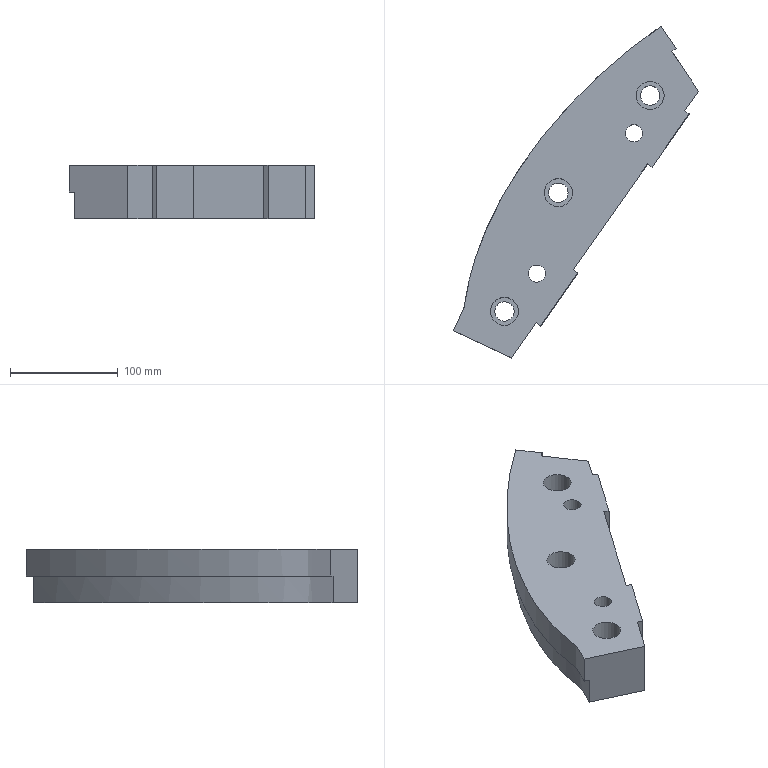Part | NX | features solid 2 | 1 solid | 29 faces | box 227.063 x 307.459 x 50 mm | volume 1256974 mm3 | plane 18 | cylinder 8 | spline 3 | commonest cylinder face diameters 18 x3 26 x3 16 x2
STEP:
#1=CARTESIAN_POINT('',(-702.221,92.253,-50.));
#2=VERTEX_POINT('',#1);
#3=CARTESIAN_POINT('',(-711.221,92.253,-50.));
#4=DIRECTION('',(0.,0.,1.));
#5=DIRECTION('',(1.,0.,0.));
#6=AXIS2_PLACEMENT_3D('',#3,#4,#5);
#7=CIRCLE('',#6,9.);
#8=EDGE_CURVE('',#2,#2,#7,.T.);
#9=ORIENTED_EDGE('',*,*,#8,.F.);
#10=EDGE_LOOP('',(#9));
#11=FACE_BOUND('',#10,.T.);
#12=CARTESIAN_POINT('',(-702.221,92.253,-30.));
#13=VERTEX_POINT('',#12);
#14=CARTESIAN_POINT('',(-711.221,92.253,-30.));
#15=DIRECTION('',(0.,0.,1.));
#16=DIRECTION('',(1.,0.,0.));
#17=AXIS2_PLACEMENT_3D('',#14,#15,#16);
#18=CIRCLE('',#17,9.);
#19=EDGE_CURVE('',#13,#13,#18,.F.);
#20=ORIENTED_EDGE('',*,*,#19,.F.);
#21=EDGE_LOOP('',(#20));
#22=FACE_BOUND('',#21,.T.);
#23=CARTESIAN_POINT('',(-711.221,92.253,-125.));
#24=DIRECTION('',(0.,0.,1.));
#25=DIRECTION('',(1.,0.,0.));
#26=AXIS2_PLACEMENT_3D('',#23,#24,#25);
#27=CYLINDRICAL_SURFACE('',#26,9.);
#28=ADVANCED_FACE('',(#11,#22),#27,.F.);
#29=CARTESIAN_POINT('',(-652.221,202.253,-50.));
#30=VERTEX_POINT('',#29);
#31=CARTESIAN_POINT('',(-661.221,202.253,-50.));
#32=DIRECTION('',(0.,0.,1.));
#33=DIRECTION('',(1.,0.,0.));
#34=AXIS2_PLACEMENT_3D('',#31,#32,#33);
#35=CIRCLE('',#34,9.);
#36=EDGE_CURVE('',#30,#30,#35,.T.);
#37=ORIENTED_EDGE('',*,*,#36,.F.);
#38=EDGE_LOOP('',(#37));
#39=FACE_BOUND('',#38,.T.);
#40=CARTESIAN_POINT('',(-652.221,202.253,-30.));
#41=VERTEX_POINT('',#40);
#42=CARTESIAN_POINT('',(-661.221,202.253,-30.));
#43=DIRECTION('',(0.,0.,1.));
#44=DIRECTION('',(1.,0.,0.));
#45=AXIS2_PLACEMENT_3D('',#42,#43,#44);
#46=CIRCLE('',#45,9.);
#47=EDGE_CURVE('',#41,#41,#46,.F.);
#48=ORIENTED_EDGE('',*,*,#47,.F.);
#49=EDGE_LOOP('',(#48));
#50=FACE_BOUND('',#49,.T.);
#51=CARTESIAN_POINT('',(-661.221,202.253,-125.));
#52=DIRECTION('',(0.,0.,1.));
#53=DIRECTION('',(1.,0.,0.));
#54=AXIS2_PLACEMENT_3D('',#51,#52,#53);
#55=CYLINDRICAL_SURFACE('',#54,9.);
#56=ADVANCED_FACE('',(#39,#50),#55,.F.);
#57=CARTESIAN_POINT('',(-567.221,292.253,-50.));
#58=VERTEX_POINT('',#57);
#59=CARTESIAN_POINT('',(-576.221,292.253,-50.));
#60=DIRECTION('',(0.,0.,1.));
#61=DIRECTION('',(1.,0.,0.));
#62=AXIS2_PLACEMENT_3D('',#59,#60,#61);
#63=CIRCLE('',#62,9.);
#64=EDGE_CURVE('',#58,#58,#63,.T.);
#65=ORIENTED_EDGE('',*,*,#64,.F.);
#66=EDGE_LOOP('',(#65));
#67=FACE_BOUND('',#66,.T.);
#68=CARTESIAN_POINT('',(-567.221,292.253,-30.));
#69=VERTEX_POINT('',#68);
#70=CARTESIAN_POINT('',(-576.221,292.253,-30.));
#71=DIRECTION('',(0.,0.,1.));
#72=DIRECTION('',(1.,0.,0.));
#73=AXIS2_PLACEMENT_3D('',#70,#71,#72);
#74=CIRCLE('',#73,9.);
#75=EDGE_CURVE('',#69,#69,#74,.F.);
#76=ORIENTED_EDGE('',*,*,#75,.F.);
#77=EDGE_LOOP('',(#76));
#78=FACE_BOUND('',#77,.T.);
#79=CARTESIAN_POINT('',(-576.221,292.253,-125.));
#80=DIRECTION('',(0.,0.,1.));
#81=DIRECTION('',(1.,0.,0.));
#82=AXIS2_PLACEMENT_3D('',#79,#80,#81);
#83=CYLINDRICAL_SURFACE('',#82,9.);
#84=ADVANCED_FACE('',(#67,#78),#83,.F.);
#85=CARTESIAN_POINT('',(-578.59,228.85,0.));
#86=VERTEX_POINT('',#85);
#87=CARTESIAN_POINT('',(-647.285,130.742,0.));
#88=VERTEX_POINT('',#87);
#89=CARTESIAN_POINT('',(-699.862,55.655,0.));
#90=DIRECTION('',(0.5736,0.8192,0.));
#91=VECTOR('',#90,1000.);
#92=LINE('',#89,#91);
#93=EDGE_CURVE('',#86,#88,#92,.F.);
#94=ORIENTED_EDGE('',*,*,#93,.T.);
#95=CARTESIAN_POINT('',(-647.285,130.742,-50.));
#96=VERTEX_POINT('',#95);
#97=CARTESIAN_POINT('',(-647.285,130.742,-70.));
#98=DIRECTION('',(0.,0.,-1.));
#99=VECTOR('',#98,1000.);
#100=LINE('',#97,#99);
#101=EDGE_CURVE('',#88,#96,#100,.T.);
#102=ORIENTED_EDGE('',*,*,#101,.T.);
#103=CARTESIAN_POINT('',(-578.59,228.85,-50.));
#104=VERTEX_POINT('',#103);
#105=CARTESIAN_POINT('',(-844.558,-150.992,-50.));
#106=DIRECTION('',(0.5736,0.8192,0.));
#107=VECTOR('',#106,1000.);
#108=LINE('',#105,#107);
#109=EDGE_CURVE('',#96,#104,#108,.T.);
#110=ORIENTED_EDGE('',*,*,#109,.T.);
#111=CARTESIAN_POINT('',(-578.59,228.85,-70.));
#112=DIRECTION('',(0.,0.,-1.));
#113=VECTOR('',#112,1000.);
#114=LINE('',#111,#113);
#115=EDGE_CURVE('',#86,#104,#114,.T.);
#116=ORIENTED_EDGE('',*,*,#115,.F.);
#117=EDGE_LOOP('',(#94,#102,#110,#116));
#118=FACE_BOUND('',#117,.T.);
#119=CARTESIAN_POINT('',(-705.68,47.346,-70.));
#120=DIRECTION('',(0.8192,-0.5736,0.));
#121=DIRECTION('',(0.5736,0.8192,0.));
#122=AXIS2_PLACEMENT_3D('',#119,#120,#121);
#123=PLANE('',#122);
#124=ADVANCED_FACE('',(#118),#123,.T.);
#125=CARTESIAN_POINT('',(-531.399,296.245,0.));
#126=VERTEX_POINT('',#125);
#127=CARTESIAN_POINT('',(-544.175,277.999,0.));
#128=VERTEX_POINT('',#127);
#129=CARTESIAN_POINT('',(-699.862,55.655,0.));
#130=DIRECTION('',(0.5736,0.8192,0.));
#131=VECTOR('',#130,1000.);
#132=LINE('',#129,#131);
#133=EDGE_CURVE('',#126,#128,#132,.F.);
#134=ORIENTED_EDGE('',*,*,#133,.T.);
#135=CARTESIAN_POINT('',(-544.175,277.999,-50.));
#136=VERTEX_POINT('',#135);
#137=CARTESIAN_POINT('',(-544.175,277.999,-70.));
#138=DIRECTION('',(0.,0.,-1.));
#139=VECTOR('',#138,1000.);
#140=LINE('',#137,#139);
#141=EDGE_CURVE('',#128,#136,#140,.T.);
#142=ORIENTED_EDGE('',*,*,#141,.T.);
#143=CARTESIAN_POINT('',(-531.399,296.245,-50.));
#144=VERTEX_POINT('',#143);
#145=CARTESIAN_POINT('',(-844.558,-150.992,-50.));
#146=DIRECTION('',(0.5736,0.8192,0.));
#147=VECTOR('',#146,1000.);
#148=LINE('',#145,#147);
#149=EDGE_CURVE('',#136,#144,#148,.T.);
#150=ORIENTED_EDGE('',*,*,#149,.T.);
#151=CARTESIAN_POINT('',(-531.399,296.245,-70.));
#152=DIRECTION('',(0.,0.,1.));
#153=VECTOR('',#152,1000.);
#154=LINE('',#151,#153);
#155=EDGE_CURVE('',#144,#126,#154,.T.);
#156=ORIENTED_EDGE('',*,*,#155,.T.);
#157=EDGE_LOOP('',(#134,#142,#150,#156));
#158=FACE_BOUND('',#157,.T.);
#159=CARTESIAN_POINT('',(-705.68,47.346,-70.));
#160=DIRECTION('',(0.8192,-0.5736,0.));
#161=DIRECTION('',(0.5736,0.8192,0.));
#162=AXIS2_PLACEMENT_3D('',#159,#160,#161);
#163=PLANE('',#162);
#164=ADVANCED_FACE('',(#158),#163,.T.);
#165=CARTESIAN_POINT('',(-567.378,349.586,-50.));
#166=VERTEX_POINT('',#165);
#167=CARTESIAN_POINT('',(-567.378,349.586,-25.));
#168=VERTEX_POINT('',#167);
#169=CARTESIAN_POINT('',(-567.378,349.586,-42.5));
#170=DIRECTION('',(0.,0.,1.));
#171=VECTOR('',#170,1000.);
#172=LINE('',#169,#171);
#173=EDGE_CURVE('',#166,#168,#172,.T.);
#174=ORIENTED_EDGE('',*,*,#173,.F.);
#175=CARTESIAN_POINT('',(-753.931,72.246,-50.));
#176=VERTEX_POINT('',#175);
#177=CARTESIAN_POINT('',(-753.931,72.246,-50.));
#178=CARTESIAN_POINT('',(-752.551,75.205,-50.));
#179=CARTESIAN_POINT('',(-750.712,79.146,-50.));
#180=CARTESIAN_POINT('',(-748.724,83.409,-50.));
#181=CARTESIAN_POINT('',(-747.464,86.109,-50.));
#182=CARTESIAN_POINT('',(-746.436,88.312,-50.));
#183=CARTESIAN_POINT('',(-745.772,89.735,-50.));
#184=CARTESIAN_POINT('',(-745.356,90.624,-50.));
#185=CARTESIAN_POINT('',(-745.145,91.076,-50.));
#186=CARTESIAN_POINT('',(-745.004,91.377,-50.));
#187=CARTESIAN_POINT('',(-744.914,91.569,-50.));
#188=CARTESIAN_POINT('',(-744.848,91.71,-50.));
#189=CARTESIAN_POINT('',(-744.815,91.781,-50.));
#190=CARTESIAN_POINT('',(-744.787,91.841,-50.));
#191=CARTESIAN_POINT('',(-744.797,91.819,-50.));
#192=CARTESIAN_POINT('',(-744.692,92.043,-50.));
#193=CARTESIAN_POINT('',(-744.597,92.252,-50.));
#194=CARTESIAN_POINT('',(-744.419,92.651,-50.));
#195=CARTESIAN_POINT('',(-744.109,93.399,-50.));
#196=CARTESIAN_POINT('',(-743.77,94.346,-50.));
#197=CARTESIAN_POINT('',(-743.446,95.594,-50.));
#198=CARTESIAN_POINT('',(-743.219,97.004,-50.));
#199=CARTESIAN_POINT('',(-743.024,98.542,-50.));
#200=CARTESIAN_POINT('',(-742.827,99.93,-50.));
#201=CARTESIAN_POINT('',(-742.634,101.268,-50.));
#202=CARTESIAN_POINT('',(-742.458,102.433,-50.));
#203=CARTESIAN_POINT('',(-742.239,103.818,-50.));
#204=CARTESIAN_POINT('',(-741.949,105.59,-50.));
#205=CARTESIAN_POINT('',(-741.559,107.839,-50.));
#206=CARTESIAN_POINT('',(-741.064,110.513,-50.));
#207=CARTESIAN_POINT('',(-740.519,113.264,-50.));
#208=CARTESIAN_POINT('',(-739.995,115.766,-50.));
#209=CARTESIAN_POINT('',(-739.238,119.196,-50.));
#210=CARTESIAN_POINT('',(-737.817,125.17,-50.));
#211=CARTESIAN_POINT('',(-735.949,132.044,-50.));
#212=CARTESIAN_POINT('',(-733.843,138.944,-50.));
#213=CARTESIAN_POINT('',(-732.145,144.128,-50.));
#214=CARTESIAN_POINT('',(-730.623,148.481,-50.));
#215=CARTESIAN_POINT('',(-729.362,151.925,-50.));
#216=CARTESIAN_POINT('',(-728.339,154.635,-50.));
#217=CARTESIAN_POINT('',(-727.468,156.882,-50.));
#218=CARTESIAN_POINT('',(-726.214,160.039,-50.));
#219=CARTESIAN_POINT('',(-724.611,163.93,-50.));
#220=CARTESIAN_POINT('',(-722.587,168.622,-50.));
#221=CARTESIAN_POINT('',(-719.77,174.869,-50.));
#222=CARTESIAN_POINT('',(-716.019,182.678,-50.));
#223=CARTESIAN_POINT('',(-711.153,192.044,-50.));
#224=CARTESIAN_POINT('',(-705.922,201.407,-50.));
#225=CARTESIAN_POINT('',(-700.323,210.77,-50.));
#226=CARTESIAN_POINT('',(-695.36,218.56,-50.));
#227=CARTESIAN_POINT('',(-691.712,224.03,-50.));
#228=CARTESIAN_POINT('',(-689.603,227.126,-50.));
#229=CARTESIAN_POINT('',(-687.94,229.531,-50.));
#230=CARTESIAN_POINT('',(-686.478,231.617,-50.));
#231=CARTESIAN_POINT('',(-684.43,234.502,-50.));
#232=CARTESIAN_POINT('',(-680.824,239.483,-50.));
#233=CARTESIAN_POINT('',(-675.492,246.575,-50.));
#234=CARTESIAN_POINT('',(-669.938,253.603,-50.));
#235=CARTESIAN_POINT('',(-665.38,259.168,-50.));
#236=CARTESIAN_POINT('',(-661.844,263.382,-50.));
#237=CARTESIAN_POINT('',(-658.443,267.345,-50.));
#238=CARTESIAN_POINT('',(-653.774,272.668,-50.));
#239=CARTESIAN_POINT('',(-647.828,279.227,-50.));
#240=CARTESIAN_POINT('',(-640.502,286.968,-50.));
#241=CARTESIAN_POINT('',(-632.883,294.678,-50.));
#242=CARTESIAN_POINT('',(-625.396,301.943,-50.));
#243=CARTESIAN_POINT('',(-615.06,311.564,-50.));
#244=CARTESIAN_POINT('',(-596.387,327.892,-50.));
#245=CARTESIAN_POINT('',(-579.271,341.12,-50.));
#246=CARTESIAN_POINT('',(-567.378,349.586,-50.));
#247=B_SPLINE_CURVE_WITH_KNOTS('',3,(#177,#178,#179,#180,#181,#182,#183,#184,#185,#186,#187,#188,#189,#190,#191,#192,#193,#194,#195,#196,#197,#198,#199,#200,#201,#202,#203,#204,#205,#206,#207,#208,#209,#210,#211,#212,#213,#214,#215,#216,#217,#218,#219,#220,#221,#222,#223,#224,#225,#226,#227,#228,#229,#230,#231,#232,#233,#234,#235,#236,#237,#238,#239,#240,#241,#242,#243,#244,#245,#246),.UNSPECIFIED.,.F.,.F.,(4,1,1,1,1,1,1,1,1,1,1,1,1,1,1,1,1,1,1,1,1,1,1,1,1,1,1,1,1,1,1,1,1,1,1,1,1,1,1,1,1,1,1,1,1,1,1,1,1,1,1,1,1,1,1,1,1,1,1,1,1,1,1,1,1,1,1,4),(0.,0.01562,0.02344,0.03125,0.03906,0.04688,0.05078,0.05469,0.05664,0.05859,0.06055,0.06152,0.06201,0.0625,0.06299,0.06348,0.06445,0.06641,0.07031,0.07422,0.07812,0.08203,0.08594,0.08984,0.09375,0.09766,0.1016,0.1094,0.1172,0.125,0.1328,0.1406,0.1562,0.1875,0.2031,0.2188,0.2344,0.2422,0.25,0.2578,0.2656,0.2812,0.2969,0.3125,0.3438,0.375,0.4062,0.4375,0.4688,0.4844,0.4922,0.5,0.5078,0.5156,0.5312,0.5625,0.5938,0.6094,0.625,0.6406,0.6562,0.6875,0.7188,0.75,0.7812,0.8125,0.875,1.),.UNSPECIFIED.);
#248=EDGE_CURVE('',#176,#166,#247,.T.);
#249=ORIENTED_EDGE('',*,*,#248,.F.);
#250=CARTESIAN_POINT('',(-753.931,72.246,-25.));
#251=VERTEX_POINT('',#250);
#252=CARTESIAN_POINT('',(-753.931,72.246,-42.5));
#253=DIRECTION('',(0.,0.,1.));
#254=VECTOR('',#253,1000.);
#255=LINE('',#252,#254);
#256=EDGE_CURVE('',#176,#251,#255,.T.);
#257=ORIENTED_EDGE('',*,*,#256,.T.);
#258=CARTESIAN_POINT('',(-567.378,349.586,-25.));
#259=CARTESIAN_POINT('',(-579.003,341.311,-25.));
#260=CARTESIAN_POINT('',(-601.651,323.884,-25.));
#261=CARTESIAN_POINT('',(-633.362,294.993,-25.));
#262=CARTESIAN_POINT('',(-657.503,268.971,-25.));
#263=CARTESIAN_POINT('',(-675.422,246.874,-25.));
#264=CARTESIAN_POINT('',(-688.122,229.581,-25.));
#265=CARTESIAN_POINT('',(-699.93,211.672,-25.));
#266=CARTESIAN_POINT('',(-710.667,193.273,-25.));
#267=CARTESIAN_POINT('',(-720.263,174.286,-25.));
#268=CARTESIAN_POINT('',(-728.596,154.68,-25.));
#269=CARTESIAN_POINT('',(-734.383,137.731,-25.));
#270=CARTESIAN_POINT('',(-738.192,123.83,-25.));
#271=CARTESIAN_POINT('',(-740.199,115.014,-25.));
#272=CARTESIAN_POINT('',(-741.571,107.876,-25.));
#273=CARTESIAN_POINT('',(-742.317,103.375,-25.));
#274=CARTESIAN_POINT('',(-742.867,99.758,-25.));
#275=CARTESIAN_POINT('',(-743.198,97.016,-25.));
#276=CARTESIAN_POINT('',(-743.685,94.33,-25.));
#277=CARTESIAN_POINT('',(-744.763,91.854,-25.));
#278=CARTESIAN_POINT('',(-745.932,89.412,-25.));
#279=CARTESIAN_POINT('',(-747.448,86.139,-25.));
#280=CARTESIAN_POINT('',(-749.358,82.054,-25.));
#281=CARTESIAN_POINT('',(-751.643,77.15,-25.));
#282=CARTESIAN_POINT('',(-753.168,73.88,-25.));
#283=CARTESIAN_POINT('',(-753.931,72.246,-25.));
#284=B_SPLINE_CURVE_WITH_KNOTS('',3,(#258,#259,#260,#261,#262,#263,#264,#265,#266,#267,#268,#269,#270,#271,#272,#273,#274,#275,#276,#277,#278,#279,#280,#281,#282,#283),.UNSPECIFIED.,.F.,.F.,(4,1,1,1,1,1,1,1,1,1,1,1,1,1,1,1,1,1,1,1,1,1,1,4),(0.7775,0.8203,0.8631,0.9059,0.9273,0.9487,0.9701,0.9916,1.013,1.034,1.056,1.066,1.077,1.083,1.088,1.091,1.093,1.096,1.099,1.101,1.104,1.109,1.115,1.12),.UNSPECIFIED.);
#285=EDGE_CURVE('',#251,#168,#284,.F.);
#286=ORIENTED_EDGE('',*,*,#285,.T.);
#287=EDGE_LOOP('',(#174,#249,#257,#286));
#288=FACE_BOUND('',#287,.T.);
#289=CARTESIAN_POINT('',(-753.931,72.246,-50.));
#290=CARTESIAN_POINT('',(-753.931,72.246,-25.));
#291=CARTESIAN_POINT('',(-753.17,73.877,-50.));
#292=CARTESIAN_POINT('',(-753.17,73.877,-25.));
#293=CARTESIAN_POINT('',(-751.649,77.139,-50.));
#294=CARTESIAN_POINT('',(-751.649,77.139,-25.));
#295=CARTESIAN_POINT('',(-749.747,81.217,-50.));
#296=CARTESIAN_POINT('',(-749.747,81.217,-25.));
#297=CARTESIAN_POINT('',(-748.226,84.48,-50.));
#298=CARTESIAN_POINT('',(-748.226,84.48,-25.));
#299=CARTESIAN_POINT('',(-747.275,86.518,-50.));
#300=CARTESIAN_POINT('',(-747.275,86.518,-25.));
#301=CARTESIAN_POINT('',(-746.514,88.151,-50.));
#302=CARTESIAN_POINT('',(-746.514,88.151,-25.));
#303=CARTESIAN_POINT('',(-745.946,89.367,-50.));
#304=CARTESIAN_POINT('',(-745.946,89.367,-25.));
#305=CARTESIAN_POINT('',(-745.367,90.611,-50.));
#306=CARTESIAN_POINT('',(-745.367,90.611,-25.));
#307=CARTESIAN_POINT('',(-744.842,91.716,-50.));
#308=CARTESIAN_POINT('',(-744.842,91.716,-25.));
#309=CARTESIAN_POINT('',(-744.099,93.332,-50.));
#310=CARTESIAN_POINT('',(-744.099,93.332,-25.));
#311=CARTESIAN_POINT('',(-743.469,95.313,-50.));
#312=CARTESIAN_POINT('',(-743.469,95.313,-25.));
#313=CARTESIAN_POINT('',(-743.227,96.983,-50.));
#314=CARTESIAN_POINT('',(-743.227,96.983,-25.));
#315=CARTESIAN_POINT('',(-743.125,97.786,-50.));
#316=CARTESIAN_POINT('',(-743.125,97.786,-25.));
#317=CARTESIAN_POINT('',(-743.005,98.675,-50.));
#318=CARTESIAN_POINT('',(-743.005,98.675,-25.));
#319=CARTESIAN_POINT('',(-742.855,99.756,-50.));
#320=CARTESIAN_POINT('',(-742.855,99.756,-25.));
#321=CARTESIAN_POINT('',(-742.601,101.501,-50.));
#322=CARTESIAN_POINT('',(-742.601,101.501,-25.));
#323=CARTESIAN_POINT('',(-742.266,103.673,-50.));
#324=CARTESIAN_POINT('',(-742.266,103.673,-25.));
#325=CARTESIAN_POINT('',(-741.833,106.278,-50.));
#326=CARTESIAN_POINT('',(-741.833,106.278,-25.));
#327=CARTESIAN_POINT('',(-741.216,109.745,-50.));
#328=CARTESIAN_POINT('',(-741.216,109.745,-25.));
#329=CARTESIAN_POINT('',(-740.369,114.065,-50.));
#330=CARTESIAN_POINT('',(-740.369,114.065,-25.));
#331=CARTESIAN_POINT('',(-739.238,119.229,-50.));
#332=CARTESIAN_POINT('',(-739.238,119.229,-25.));
#333=CARTESIAN_POINT('',(-737.579,126.085,-50.));
#334=CARTESIAN_POINT('',(-737.579,126.085,-25.));
#335=CARTESIAN_POINT('',(-735.232,134.596,-50.));
#336=CARTESIAN_POINT('',(-735.232,134.596,-25.));
#337=CARTESIAN_POINT('',(-732.002,144.701,-50.));
#338=CARTESIAN_POINT('',(-732.002,144.701,-25.));
#339=CARTESIAN_POINT('',(-727.177,158.017,-50.));
#340=CARTESIAN_POINT('',(-727.177,158.017,-25.));
#341=CARTESIAN_POINT('',(-720.244,174.327,-50.));
#342=CARTESIAN_POINT('',(-720.244,174.327,-25.));
#343=CARTESIAN_POINT('',(-710.641,193.322,-50.));
#344=CARTESIAN_POINT('',(-710.641,193.322,-25.));
#345=CARTESIAN_POINT('',(-699.889,211.737,-50.));
#346=CARTESIAN_POINT('',(-699.889,211.737,-25.));
#347=CARTESIAN_POINT('',(-684.216,235.503,-50.));
#348=CARTESIAN_POINT('',(-684.216,235.503,-25.));
#349=CARTESIAN_POINT('',(-662.409,263.684,-50.));
#350=CARTESIAN_POINT('',(-662.409,263.684,-25.));
#351=CARTESIAN_POINT('',(-623.582,305.544,-50.));
#352=CARTESIAN_POINT('',(-623.582,305.544,-25.));
#353=CARTESIAN_POINT('',(-590.637,333.029,-50.));
#354=CARTESIAN_POINT('',(-590.637,333.029,-25.));
#355=CARTESIAN_POINT('',(-567.378,349.586,-50.));
#356=CARTESIAN_POINT('',(-567.378,349.586,-25.));
#357=B_SPLINE_SURFACE_WITH_KNOTS('',3,1,((#289,#290),(#291,#292),(#293,#294),(#295,#296),(#297,#298),(#299,#300),(#301,#302),(#303,#304),(#305,#306),(#307,#308),(#309,#310),(#311,#312),(#313,#314),(#315,#316),(#317,#318),(#319,#320),(#321,#322),(#323,#324),(#325,#326),(#327,#328),(#329,#330),(#331,#332),(#333,#334),(#335,#336),(#337,#338),(#339,#340),(#341,#342),(#343,#344),(#345,#346),(#347,#348),(#349,#350),(#351,#352),(#353,#354),(#355,#356)),.SURF_OF_LINEAR_EXTRUSION.,.F.,.F.,.F.,(4,1,1,1,1,1,1,1,1,1,1,1,1,1,1,1,1,1,1,1,1,1,1,1,1,1,1,1,1,1,1,4),(2,2),(0.,0.0154,0.03079,0.03849,0.04619,0.05004,0.05389,0.05774,0.06159,0.06544,0.06928,0.07313,0.07506,0.07698,0.08083,0.08468,0.09238,0.1001,0.1078,0.1232,0.1386,0.154,0.1848,0.2156,0.2463,0.3079,0.3695,0.4311,0.4927,0.6159,0.739,0.9854),(0.,1.),.UNSPECIFIED.);
#358=ADVANCED_FACE('',(#288),#357,.F.);
#359=CARTESIAN_POINT('',(-704.413,49.155,-50.));
#360=VERTEX_POINT('',#359);
#361=CARTESIAN_POINT('',(-704.413,49.155,0.));
#362=VERTEX_POINT('',#361);
#363=CARTESIAN_POINT('',(-704.413,49.155,-70.));
#364=DIRECTION('',(0.,0.,1.));
#365=VECTOR('',#364,1000.);
#366=LINE('',#363,#365);
#367=EDGE_CURVE('',#360,#362,#366,.T.);
#368=ORIENTED_EDGE('',*,*,#367,.F.);
#369=CARTESIAN_POINT('',(-681.7,81.593,-50.));
#370=VERTEX_POINT('',#369);
#371=CARTESIAN_POINT('',(-844.558,-150.992,-50.));
#372=DIRECTION('',(0.5736,0.8192,0.));
#373=VECTOR('',#372,1000.);
#374=LINE('',#371,#373);
#375=EDGE_CURVE('',#360,#370,#374,.T.);
#376=ORIENTED_EDGE('',*,*,#375,.T.);
#377=CARTESIAN_POINT('',(-681.7,81.593,0.));
#378=VERTEX_POINT('',#377);
#379=CARTESIAN_POINT('',(-681.7,81.593,-70.));
#380=DIRECTION('',(0.,0.,-1.));
#381=VECTOR('',#380,1000.);
#382=LINE('',#379,#381);
#383=EDGE_CURVE('',#378,#370,#382,.T.);
#384=ORIENTED_EDGE('',*,*,#383,.F.);
#385=CARTESIAN_POINT('',(-699.862,55.655,0.));
#386=DIRECTION('',(0.5736,0.8192,0.));
#387=VECTOR('',#386,1000.);
#388=LINE('',#385,#387);
#389=EDGE_CURVE('',#378,#362,#388,.F.);
#390=ORIENTED_EDGE('',*,*,#389,.T.);
#391=EDGE_LOOP('',(#368,#376,#384,#390));
#392=FACE_BOUND('',#391,.T.);
#393=CARTESIAN_POINT('',(-705.68,47.346,-70.));
#394=DIRECTION('',(0.8192,-0.5736,0.));
#395=DIRECTION('',(0.5736,0.8192,0.));
#396=AXIS2_PLACEMENT_3D('',#393,#394,#395);
#397=PLANE('',#396);
#398=ADVANCED_FACE('',(#392),#397,.T.);
#399=CARTESIAN_POINT('',(-552.106,335.885,-25.));
#400=VERTEX_POINT('',#399);
#401=CARTESIAN_POINT('',(-552.106,335.885,0.));
#402=VERTEX_POINT('',#401);
#403=CARTESIAN_POINT('',(-552.106,335.885,-12.5));
#404=DIRECTION('',(0.,0.,-1.));
#405=VECTOR('',#404,1000.);
#406=LINE('',#403,#405);
#407=EDGE_CURVE('',#400,#402,#406,.F.);
#408=ORIENTED_EDGE('',*,*,#407,.F.);
#409=CARTESIAN_POINT('',(-566.088,356.614,-25.));
#410=VERTEX_POINT('',#409);
#411=CARTESIAN_POINT('',(822.371,-1701.861,-25.));
#412=DIRECTION('',(-0.5592,0.829,0.));
#413=VECTOR('',#412,1000.);
#414=LINE('',#411,#413);
#415=EDGE_CURVE('',#400,#410,#414,.T.);
#416=ORIENTED_EDGE('',*,*,#415,.T.);
#417=CARTESIAN_POINT('',(-566.088,356.614,0.));
#418=VERTEX_POINT('',#417);
#419=CARTESIAN_POINT('',(-566.088,356.614,-70.));
#420=DIRECTION('',(0.,0.,1.));
#421=VECTOR('',#420,1000.);
#422=LINE('',#419,#421);
#423=EDGE_CURVE('',#410,#418,#422,.T.);
#424=ORIENTED_EDGE('',*,*,#423,.T.);
#425=CARTESIAN_POINT('',(822.371,-1701.861,0.));
#426=DIRECTION('',(0.5592,-0.829,0.));
#427=VECTOR('',#426,1000.);
#428=LINE('',#425,#427);
#429=EDGE_CURVE('',#402,#418,#428,.F.);
#430=ORIENTED_EDGE('',*,*,#429,.F.);
#431=EDGE_LOOP('',(#408,#416,#424,#430));
#432=FACE_BOUND('',#431,.T.);
#433=CARTESIAN_POINT('',(822.371,-1701.861,-70.));
#434=DIRECTION('',(0.829,0.5592,0.));
#435=DIRECTION('',(-0.5592,0.829,0.));
#436=AXIS2_PLACEMENT_3D('',#433,#434,#435);
#437=PLANE('',#436);
#438=ADVANCED_FACE('',(#432),#437,.T.);
#439=ORIENTED_EDGE('',*,*,#8,.T.);
#440=EDGE_LOOP('',(#439));
#441=FACE_BOUND('',#440,.T.);
#442=CARTESIAN_POINT('',(-673.221,127.253,-50.));
#443=VERTEX_POINT('',#442);
#444=CARTESIAN_POINT('',(-681.221,127.253,-50.));
#445=DIRECTION('',(0.,0.,1.));
#446=DIRECTION('',(1.,0.,0.));
#447=AXIS2_PLACEMENT_3D('',#444,#445,#446);
#448=CIRCLE('',#447,8.);
#449=EDGE_CURVE('',#443,#443,#448,.T.);
#450=ORIENTED_EDGE('',*,*,#449,.T.);
#451=EDGE_LOOP('',(#450));
#452=FACE_BOUND('',#451,.T.);
#453=ORIENTED_EDGE('',*,*,#36,.T.);
#454=EDGE_LOOP('',(#453));
#455=FACE_BOUND('',#454,.T.);
#456=CARTESIAN_POINT('',(-583.221,257.253,-50.));
#457=VERTEX_POINT('',#456);
#458=CARTESIAN_POINT('',(-591.221,257.253,-50.));
#459=DIRECTION('',(0.,0.,1.));
#460=DIRECTION('',(1.,0.,0.));
#461=AXIS2_PLACEMENT_3D('',#458,#459,#460);
#462=CIRCLE('',#461,8.);
#463=EDGE_CURVE('',#457,#457,#462,.T.);
#464=ORIENTED_EDGE('',*,*,#463,.T.);
#465=EDGE_LOOP('',(#464));
#466=FACE_BOUND('',#465,.T.);
#467=ORIENTED_EDGE('',*,*,#64,.T.);
#468=EDGE_LOOP('',(#467));
#469=FACE_BOUND('',#468,.T.);
#470=ORIENTED_EDGE('',*,*,#375,.F.);
#471=CARTESIAN_POINT('',(-752.052,71.37,-50.));
#472=DIRECTION('',(0.9063,-0.4226,0.));
#473=VECTOR('',#472,1000.);
#474=LINE('',#471,#473);
#475=EDGE_CURVE('',#176,#360,#474,.T.);
#476=ORIENTED_EDGE('',*,*,#475,.F.);
#477=ORIENTED_EDGE('',*,*,#248,.T.);
#478=CARTESIAN_POINT('',(-427.361,142.001,-50.));
#479=DIRECTION('',(-0.5592,0.829,0.));
#480=VECTOR('',#479,1000.);
#481=LINE('',#478,#480);
#482=EDGE_CURVE('',#144,#166,#481,.T.);
#483=ORIENTED_EDGE('',*,*,#482,.F.);
#484=ORIENTED_EDGE('',*,*,#149,.F.);
#485=CARTESIAN_POINT('',(-540.079,275.131,-50.));
#486=VERTEX_POINT('',#485);
#487=CARTESIAN_POINT('',(-527.792,266.527,-50.));
#488=DIRECTION('',(0.8192,-0.5736,0.));
#489=VECTOR('',#488,1000.);
#490=LINE('',#487,#489);
#491=EDGE_CURVE('',#136,#486,#490,.T.);
#492=ORIENTED_EDGE('',*,*,#491,.T.);
#493=CARTESIAN_POINT('',(-574.494,225.982,-50.));
#494=VERTEX_POINT('',#493);
#495=CARTESIAN_POINT('',(-840.462,-153.86,-50.));
#496=DIRECTION('',(0.5736,0.8192,0.));
#497=VECTOR('',#496,1000.);
#498=LINE('',#495,#497);
#499=EDGE_CURVE('',#494,#486,#498,.T.);
#500=ORIENTED_EDGE('',*,*,#499,.F.);
#501=CARTESIAN_POINT('',(-562.206,217.378,-50.));
#502=DIRECTION('',(0.8192,-0.5736,0.));
#503=VECTOR('',#502,1000.);
#504=LINE('',#501,#503);
#505=EDGE_CURVE('',#104,#494,#504,.T.);
#506=ORIENTED_EDGE('',*,*,#505,.F.);
#507=ORIENTED_EDGE('',*,*,#109,.F.);
#508=CARTESIAN_POINT('',(-643.19,127.874,-50.));
#509=VERTEX_POINT('',#508);
#510=CARTESIAN_POINT('',(-630.902,119.27,-50.));
#511=DIRECTION('',(0.8192,-0.5736,0.));
#512=VECTOR('',#511,1000.);
#513=LINE('',#510,#512);
#514=EDGE_CURVE('',#96,#509,#513,.T.);
#515=ORIENTED_EDGE('',*,*,#514,.T.);
#516=CARTESIAN_POINT('',(-677.604,78.725,-50.));
#517=VERTEX_POINT('',#516);
#518=CARTESIAN_POINT('',(-840.462,-153.86,-50.));
#519=DIRECTION('',(0.5736,0.8192,0.));
#520=VECTOR('',#519,1000.);
#521=LINE('',#518,#520);
#522=EDGE_CURVE('',#517,#509,#521,.T.);
#523=ORIENTED_EDGE('',*,*,#522,.F.);
#524=CARTESIAN_POINT('',(-665.317,70.121,-50.));
#525=DIRECTION('',(0.8192,-0.5736,0.));
#526=VECTOR('',#525,1000.);
#527=LINE('',#524,#526);
#528=EDGE_CURVE('',#370,#517,#527,.T.);
#529=ORIENTED_EDGE('',*,*,#528,.F.);
#530=EDGE_LOOP('',(#470,#476,#477,#483,#484,#492,#500,#506,#507,#515,#523,#529));
#531=FACE_BOUND('',#530,.T.);
#532=CARTESIAN_POINT('',(-852.989,-145.089,-50.));
#533=DIRECTION('',(0.,0.,1.));
#534=DIRECTION('',(1.,0.,0.));
#535=AXIS2_PLACEMENT_3D('',#532,#533,#534);
#536=PLANE('',#535);
#537=ADVANCED_FACE('',(#441,#452,#455,#466,#469,#531),#536,.F.);
#538=CARTESIAN_POINT('',(-758.462,74.359,0.));
#539=VERTEX_POINT('',#538);
#540=CARTESIAN_POINT('',(-2805.507,1028.912,0.));
#541=DIRECTION('',(-0.9063,0.4226,0.));
#542=VECTOR('',#541,1000.);
#543=LINE('',#540,#542);
#544=EDGE_CURVE('',#539,#362,#543,.F.);
#545=ORIENTED_EDGE('',*,*,#544,.T.);
#546=ORIENTED_EDGE('',*,*,#389,.F.);
#547=CARTESIAN_POINT('',(-677.604,78.725,0.));
#548=VERTEX_POINT('',#547);
#549=CARTESIAN_POINT('',(-735.627,119.353,0.));
#550=DIRECTION('',(0.8192,-0.5736,0.));
#551=VECTOR('',#550,1000.);
#552=LINE('',#549,#551);
#553=EDGE_CURVE('',#378,#548,#552,.T.);
#554=ORIENTED_EDGE('',*,*,#553,.T.);
#555=CARTESIAN_POINT('',(-643.19,127.874,0.));
#556=VERTEX_POINT('',#555);
#557=CARTESIAN_POINT('',(-683.34,70.533,0.));
#558=DIRECTION('',(-0.5736,-0.8192,0.));
#559=VECTOR('',#558,1000.);
#560=LINE('',#557,#559);
#561=EDGE_CURVE('',#548,#556,#560,.F.);
#562=ORIENTED_EDGE('',*,*,#561,.T.);
#563=CARTESIAN_POINT('',(-701.212,168.502,0.));
#564=DIRECTION('',(0.8192,-0.5736,0.));
#565=VECTOR('',#564,1000.);
#566=LINE('',#563,#565);
#567=EDGE_CURVE('',#88,#556,#566,.T.);
#568=ORIENTED_EDGE('',*,*,#567,.F.);
#569=ORIENTED_EDGE('',*,*,#93,.F.);
#570=CARTESIAN_POINT('',(-574.494,225.982,0.));
#571=VERTEX_POINT('',#570);
#572=CARTESIAN_POINT('',(-632.516,266.61,0.));
#573=DIRECTION('',(0.8192,-0.5736,0.));
#574=VECTOR('',#573,1000.);
#575=LINE('',#572,#574);
#576=EDGE_CURVE('',#86,#571,#575,.T.);
#577=ORIENTED_EDGE('',*,*,#576,.T.);
#578=CARTESIAN_POINT('',(-540.079,275.131,0.));
#579=VERTEX_POINT('',#578);
#580=CARTESIAN_POINT('',(-563.022,242.365,0.));
#581=DIRECTION('',(-0.5736,-0.8192,0.));
#582=VECTOR('',#581,1000.);
#583=LINE('',#580,#582);
#584=EDGE_CURVE('',#571,#579,#583,.F.);
#585=ORIENTED_EDGE('',*,*,#584,.T.);
#586=CARTESIAN_POINT('',(-598.102,315.759,0.));
#587=DIRECTION('',(0.8192,-0.5736,0.));
#588=VECTOR('',#587,1000.);
#589=LINE('',#586,#588);
#590=EDGE_CURVE('',#128,#579,#589,.T.);
#591=ORIENTED_EDGE('',*,*,#590,.F.);
#592=ORIENTED_EDGE('',*,*,#133,.F.);
#593=CARTESIAN_POINT('',(-556.191,333.,0.));
#594=VERTEX_POINT('',#593);
#595=CARTESIAN_POINT('',(-509.098,263.181,0.));
#596=DIRECTION('',(-0.5592,0.829,0.));
#597=VECTOR('',#596,1000.);
#598=LINE('',#595,#597);
#599=EDGE_CURVE('',#126,#594,#598,.T.);
#600=ORIENTED_EDGE('',*,*,#599,.T.);
#601=CARTESIAN_POINT('',(-556.191,333.,0.));
#602=CARTESIAN_POINT('',(-554.834,333.967,0.));
#603=CARTESIAN_POINT('',(-553.472,334.93,0.));
#604=CARTESIAN_POINT('',(-552.106,335.885,0.));
#605=B_SPLINE_CURVE_WITH_KNOTS('',3,(#601,#602,#603,#604),.UNSPECIFIED.,.F.,.F.,(4,4),(1.826,1.831),.UNSPECIFIED.);
#606=EDGE_CURVE('',#594,#402,#605,.T.);
#607=ORIENTED_EDGE('',*,*,#606,.T.);
#608=ORIENTED_EDGE('',*,*,#429,.T.);
#609=CARTESIAN_POINT('',(-758.462,74.359,0.));
#610=CARTESIAN_POINT('',(-757.693,76.008,0.));
#611=CARTESIAN_POINT('',(-756.154,79.307,0.));
#612=CARTESIAN_POINT('',(-753.849,84.257,0.));
#613=CARTESIAN_POINT('',(-751.918,88.376,0.));
#614=CARTESIAN_POINT('',(-750.397,91.683,0.));
#615=CARTESIAN_POINT('',(-749.188,94.133,0.));
#616=CARTESIAN_POINT('',(-748.211,96.686,0.));
#617=CARTESIAN_POINT('',(-747.963,99.564,0.));
#618=CARTESIAN_POINT('',(-747.525,102.357,0.));
#619=CARTESIAN_POINT('',(-746.662,107.949,0.));
#620=CARTESIAN_POINT('',(-745.091,116.214,0.));
#621=CARTESIAN_POINT('',(-742.538,127.03,0.));
#622=CARTESIAN_POINT('',(-739.538,137.646,0.));
#623=CARTESIAN_POINT('',(-736.129,148.08,0.));
#624=CARTESIAN_POINT('',(-731.068,161.763,0.));
#625=CARTESIAN_POINT('',(-723.835,178.462,0.));
#626=CARTESIAN_POINT('',(-713.833,197.913,0.));
#627=CARTESIAN_POINT('',(-702.617,216.817,0.));
#628=CARTESIAN_POINT('',(-686.151,241.379,0.));
#629=CARTESIAN_POINT('',(-663.608,269.984,0.));
#630=CARTESIAN_POINT('',(-623.873,312.129,0.));
#631=CARTESIAN_POINT('',(-590.167,339.79,0.));
#632=CARTESIAN_POINT('',(-566.088,356.614,0.));
#633=B_SPLINE_CURVE_WITH_KNOTS('',3,(#609,#610,#611,#612,#613,#614,#615,#616,#617,#618,#619,#620,#621,#622,#623,#624,#625,#626,#627,#628,#629,#630,#631,#632),.UNSPECIFIED.,.F.,.F.,(4,1,1,1,1,1,1,1,1,1,1,1,1,1,1,1,1,1,1,1,1,4),(1.698,1.704,1.709,1.715,1.718,1.72,1.723,1.726,1.728,1.731,1.742,1.753,1.764,1.775,1.786,1.808,1.83,1.851,1.873,1.917,1.961,2.048),.UNSPECIFIED.);
#634=EDGE_CURVE('',#539,#418,#633,.T.);
#635=ORIENTED_EDGE('',*,*,#634,.F.);
#636=EDGE_LOOP('',(#545,#546,#554,#562,#568,#569,#577,#585,#591,#592,#600,#607,#608,#635));
#637=FACE_BOUND('',#636,.T.);
#638=CARTESIAN_POINT('',(-698.221,92.253,0.));
#639=VERTEX_POINT('',#638);
#640=CARTESIAN_POINT('',(-711.221,92.253,0.));
#641=DIRECTION('',(0.,0.,1.));
#642=DIRECTION('',(1.,0.,0.));
#643=AXIS2_PLACEMENT_3D('',#640,#641,#642);
#644=CIRCLE('',#643,13.);
#645=EDGE_CURVE('',#639,#639,#644,.T.);
#646=ORIENTED_EDGE('',*,*,#645,.F.);
#647=EDGE_LOOP('',(#646));
#648=FACE_BOUND('',#647,.T.);
#649=CARTESIAN_POINT('',(-648.221,202.253,0.));
#650=VERTEX_POINT('',#649);
#651=CARTESIAN_POINT('',(-661.221,202.253,0.));
#652=DIRECTION('',(0.,0.,1.));
#653=DIRECTION('',(1.,0.,0.));
#654=AXIS2_PLACEMENT_3D('',#651,#652,#653);
#655=CIRCLE('',#654,13.);
#656=EDGE_CURVE('',#650,#650,#655,.T.);
#657=ORIENTED_EDGE('',*,*,#656,.F.);
#658=EDGE_LOOP('',(#657));
#659=FACE_BOUND('',#658,.T.);
#660=CARTESIAN_POINT('',(-563.221,292.253,0.));
#661=VERTEX_POINT('',#660);
#662=CARTESIAN_POINT('',(-576.221,292.253,0.));
#663=DIRECTION('',(0.,0.,1.));
#664=DIRECTION('',(1.,0.,0.));
#665=AXIS2_PLACEMENT_3D('',#662,#663,#664);
#666=CIRCLE('',#665,13.);
#667=EDGE_CURVE('',#661,#661,#666,.T.);
#668=ORIENTED_EDGE('',*,*,#667,.F.);
#669=EDGE_LOOP('',(#668));
#670=FACE_BOUND('',#669,.T.);
#671=CARTESIAN_POINT('',(-673.221,127.253,0.));
#672=VERTEX_POINT('',#671);
#673=CARTESIAN_POINT('',(-681.221,127.253,0.));
#674=DIRECTION('',(0.,0.,1.));
#675=DIRECTION('',(1.,0.,0.));
#676=AXIS2_PLACEMENT_3D('',#673,#674,#675);
#677=CIRCLE('',#676,8.);
#678=EDGE_CURVE('',#672,#672,#677,.T.);
#679=ORIENTED_EDGE('',*,*,#678,.F.);
#680=EDGE_LOOP('',(#679));
#681=FACE_BOUND('',#680,.T.);
#682=CARTESIAN_POINT('',(-583.221,257.253,0.));
#683=VERTEX_POINT('',#682);
#684=CARTESIAN_POINT('',(-591.221,257.253,0.));
#685=DIRECTION('',(0.,0.,1.));
#686=DIRECTION('',(1.,0.,0.));
#687=AXIS2_PLACEMENT_3D('',#684,#685,#686);
#688=CIRCLE('',#687,8.);
#689=EDGE_CURVE('',#683,#683,#688,.T.);
#690=ORIENTED_EDGE('',*,*,#689,.F.);
#691=EDGE_LOOP('',(#690));
#692=FACE_BOUND('',#691,.T.);
#693=CARTESIAN_POINT('',(-663.,29.844,0.));
#694=DIRECTION('',(0.,0.,1.));
#695=DIRECTION('',(0.5736,0.8192,0.));
#696=AXIS2_PLACEMENT_3D('',#693,#694,#695);
#697=PLANE('',#696);
#698=ADVANCED_FACE('',(#637,#648,#659,#670,#681,#692),#697,.T.);
#699=CARTESIAN_POINT('',(-758.462,74.359,-25.));
#700=VERTEX_POINT('',#699);
#701=CARTESIAN_POINT('',(-758.462,74.359,-25.));
#702=CARTESIAN_POINT('',(-757.695,76.003,-25.));
#703=CARTESIAN_POINT('',(-756.161,79.292,-25.));
#704=CARTESIAN_POINT('',(-753.863,84.227,-25.));
#705=CARTESIAN_POINT('',(-751.938,88.335,-25.));
#706=CARTESIAN_POINT('',(-750.42,91.631,-25.));
#707=CARTESIAN_POINT('',(-749.22,94.076,-25.));
#708=CARTESIAN_POINT('',(-748.223,96.611,-25.));
#709=CARTESIAN_POINT('',(-747.973,99.481,-25.));
#710=CARTESIAN_POINT('',(-747.538,102.268,-25.));
#711=CARTESIAN_POINT('',(-746.68,107.846,-25.));
#712=CARTESIAN_POINT('',(-745.117,116.09,-25.));
#713=CARTESIAN_POINT('',(-742.577,126.879,-25.));
#714=CARTESIAN_POINT('',(-739.592,137.469,-25.));
#715=CARTESIAN_POINT('',(-736.199,147.877,-25.));
#716=CARTESIAN_POINT('',(-731.163,161.525,-25.));
#717=CARTESIAN_POINT('',(-723.966,178.181,-25.));
#718=CARTESIAN_POINT('',(-714.013,197.585,-25.));
#719=CARTESIAN_POINT('',(-702.859,216.433,-25.));
#720=CARTESIAN_POINT('',(-690.555,234.835,-25.));
#721=CARTESIAN_POINT('',(-677.333,252.572,-25.));
#722=CARTESIAN_POINT('',(-658.761,275.124,-25.));
#723=CARTESIAN_POINT('',(-633.84,301.556,-25.));
#724=CARTESIAN_POINT('',(-601.406,330.599,-25.));
#725=CARTESIAN_POINT('',(-578.115,348.211,-25.));
#726=CARTESIAN_POINT('',(-566.088,356.614,-25.));
#727=B_SPLINE_CURVE_WITH_KNOTS('',3,(#701,#702,#703,#704,#705,#706,#707,#708,#709,#710,#711,#712,#713,#714,#715,#716,#717,#718,#719,#720,#721,#722,#723,#724,#725,#726),.UNSPECIFIED.,.F.,.F.,(4,1,1,1,1,1,1,1,1,1,1,1,1,1,1,1,1,1,1,1,1,1,1,4),(1.367,1.372,1.378,1.383,1.386,1.389,1.392,1.394,1.397,1.4,1.411,1.421,1.432,1.443,1.454,1.476,1.498,1.519,1.541,1.563,1.585,1.628,1.672,1.715),.UNSPECIFIED.);
#728=EDGE_CURVE('',#700,#410,#727,.T.);
#729=ORIENTED_EDGE('',*,*,#728,.F.);
#730=CARTESIAN_POINT('',(-758.462,74.359,-2.5));
#731=DIRECTION('',(0.,0.,1.));
#732=VECTOR('',#731,1000.);
#733=LINE('',#730,#732);
#734=EDGE_CURVE('',#700,#539,#733,.T.);
#735=ORIENTED_EDGE('',*,*,#734,.T.);
#736=ORIENTED_EDGE('',*,*,#634,.T.);
#737=ORIENTED_EDGE('',*,*,#423,.F.);
#738=EDGE_LOOP('',(#729,#735,#736,#737));
#739=FACE_BOUND('',#738,.T.);
#740=CARTESIAN_POINT('',(-758.462,74.359,-25.));
#741=CARTESIAN_POINT('',(-758.462,74.359,0.));
#742=CARTESIAN_POINT('',(-757.69,76.014,-25.));
#743=CARTESIAN_POINT('',(-757.69,76.014,0.));
#744=CARTESIAN_POINT('',(-756.146,79.325,-25.));
#745=CARTESIAN_POINT('',(-756.146,79.325,0.));
#746=CARTESIAN_POINT('',(-753.833,84.292,-25.));
#747=CARTESIAN_POINT('',(-753.833,84.292,0.));
#748=CARTESIAN_POINT('',(-751.894,88.426,-25.));
#749=CARTESIAN_POINT('',(-751.894,88.426,0.));
#750=CARTESIAN_POINT('',(-750.368,91.746,-25.));
#751=CARTESIAN_POINT('',(-750.368,91.746,0.));
#752=CARTESIAN_POINT('',(-749.156,94.202,-25.));
#753=CARTESIAN_POINT('',(-749.156,94.202,0.));
#754=CARTESIAN_POINT('',(-748.335,96.346,-25.));
#755=CARTESIAN_POINT('',(-748.335,96.346,0.));
#756=CARTESIAN_POINT('',(-748.122,98.166,-25.));
#757=CARTESIAN_POINT('',(-748.122,98.166,0.));
#758=CARTESIAN_POINT('',(-747.749,100.878,-25.));
#759=CARTESIAN_POINT('',(-747.749,100.878,0.));
#760=CARTESIAN_POINT('',(-746.875,106.749,-25.));
#761=CARTESIAN_POINT('',(-746.875,106.749,0.));
#762=CARTESIAN_POINT('',(-745.194,115.721,-25.));
#763=CARTESIAN_POINT('',(-745.194,115.721,0.));
#764=CARTESIAN_POINT('',(-742.701,126.389,-25.));
#765=CARTESIAN_POINT('',(-742.701,126.389,0.));
#766=CARTESIAN_POINT('',(-739.751,136.946,-25.));
#767=CARTESIAN_POINT('',(-739.751,136.946,0.));
#768=CARTESIAN_POINT('',(-736.373,147.378,-25.));
#769=CARTESIAN_POINT('',(-736.373,147.378,0.));
#770=CARTESIAN_POINT('',(-731.333,161.108,-25.));
#771=CARTESIAN_POINT('',(-731.333,161.108,0.));
#772=CARTESIAN_POINT('',(-724.106,177.894,-25.));
#773=CARTESIAN_POINT('',(-724.106,177.894,0.));
#774=CARTESIAN_POINT('',(-710.781,203.911,-25.));
#775=CARTESIAN_POINT('',(-710.781,203.911,0.));
#776=CARTESIAN_POINT('',(-691.218,234.848,-25.));
#777=CARTESIAN_POINT('',(-691.218,234.848,0.));
#778=CARTESIAN_POINT('',(-664.149,269.379,-25.));
#779=CARTESIAN_POINT('',(-664.149,269.379,0.));
#780=CARTESIAN_POINT('',(-624.057,312.004,-25.));
#781=CARTESIAN_POINT('',(-624.057,312.004,0.));
#782=CARTESIAN_POINT('',(-590.047,339.875,-25.));
#783=CARTESIAN_POINT('',(-590.047,339.875,0.));
#784=CARTESIAN_POINT('',(-566.088,356.614,-25.));
#785=CARTESIAN_POINT('',(-566.088,356.614,0.));
#786=B_SPLINE_SURFACE_WITH_KNOTS('',3,1,((#740,#741),(#742,#743),(#744,#745),(#746,#747),(#748,#749),(#750,#751),(#752,#753),(#754,#755),(#756,#757),(#758,#759),(#760,#761),(#762,#763),(#764,#765),(#766,#767),(#768,#769),(#770,#771),(#772,#773),(#774,#775),(#776,#777),(#778,#779),(#780,#781),(#782,#783),(#784,#785)),.SURF_OF_LINEAR_EXTRUSION.,.F.,.F.,.F.,(4,1,1,1,1,1,1,1,1,1,1,1,1,1,1,1,1,1,1,1,4),(2,2),(0.003106,0.007784,0.01246,0.01714,0.01948,0.02182,0.02416,0.02533,0.02649,0.03117,0.04053,0.04988,0.05924,0.06859,0.07795,0.09666,0.1154,0.1528,0.1902,0.2276,0.3025),(0.,1.),.UNSPECIFIED.);
#787=ADVANCED_FACE('',(#739),#786,.F.);
#788=ORIENTED_EDGE('',*,*,#475,.T.);
#789=ORIENTED_EDGE('',*,*,#367,.T.);
#790=ORIENTED_EDGE('',*,*,#544,.F.);
#791=ORIENTED_EDGE('',*,*,#734,.F.);
#792=CARTESIAN_POINT('',(-758.462,74.359,-25.));
#793=DIRECTION('',(-0.9063,0.4226,0.));
#794=VECTOR('',#793,1000.);
#795=LINE('',#792,#794);
#796=EDGE_CURVE('',#251,#700,#795,.T.);
#797=ORIENTED_EDGE('',*,*,#796,.F.);
#798=ORIENTED_EDGE('',*,*,#256,.F.);
#799=EDGE_LOOP('',(#788,#789,#790,#791,#797,#798));
#800=FACE_BOUND('',#799,.T.);
#801=CARTESIAN_POINT('',(-2805.507,1028.912,-70.));
#802=DIRECTION('',(-0.4226,-0.9063,0.));
#803=DIRECTION('',(0.9063,-0.4226,0.));
#804=AXIS2_PLACEMENT_3D('',#801,#802,#803);
#805=PLANE('',#804);
#806=ADVANCED_FACE('',(#800),#805,.T.);
#807=ORIENTED_EDGE('',*,*,#415,.F.);
#808=CARTESIAN_POINT('',(-556.191,333.,-25.));
#809=VERTEX_POINT('',#808);
#810=CARTESIAN_POINT('',(-556.191,333.,-25.));
#811=CARTESIAN_POINT('',(-554.834,333.967,-25.));
#812=CARTESIAN_POINT('',(-553.473,334.929,-25.));
#813=CARTESIAN_POINT('',(-552.106,335.885,-25.));
#814=B_SPLINE_CURVE_WITH_KNOTS('',3,(#810,#811,#812,#813),.UNSPECIFIED.,.F.,.F.,(4,4),(0.9824,0.9987),.UNSPECIFIED.);
#815=EDGE_CURVE('',#809,#400,#814,.T.);
#816=ORIENTED_EDGE('',*,*,#815,.F.);
#817=CARTESIAN_POINT('',(-505.519,257.875,-25.));
#818=DIRECTION('',(-0.5592,0.829,0.));
#819=VECTOR('',#818,1000.);
#820=LINE('',#817,#819);
#821=EDGE_CURVE('',#809,#168,#820,.T.);
#822=ORIENTED_EDGE('',*,*,#821,.T.);
#823=ORIENTED_EDGE('',*,*,#285,.F.);
#824=ORIENTED_EDGE('',*,*,#796,.T.);
#825=ORIENTED_EDGE('',*,*,#728,.T.);
#826=EDGE_LOOP('',(#807,#816,#822,#823,#824,#825));
#827=FACE_BOUND('',#826,.T.);
#828=CARTESIAN_POINT('',(-758.462,74.359,-25.));
#829=DIRECTION('',(0.,0.,-1.));
#830=DIRECTION('',(-1.,0.,0.));
#831=AXIS2_PLACEMENT_3D('',#828,#829,#830);
#832=PLANE('',#831);
#833=ADVANCED_FACE('',(#827),#832,.T.);
#834=ORIENTED_EDGE('',*,*,#606,.F.);
#835=CARTESIAN_POINT('',(-556.191,333.,-25.));
#836=DIRECTION('',(0.,0.,-1.));
#837=VECTOR('',#836,1000.);
#838=LINE('',#835,#837);
#839=EDGE_CURVE('',#809,#594,#838,.F.);
#840=ORIENTED_EDGE('',*,*,#839,.F.);
#841=ORIENTED_EDGE('',*,*,#815,.T.);
#842=ORIENTED_EDGE('',*,*,#407,.T.);
#843=EDGE_LOOP('',(#834,#840,#841,#842));
#844=FACE_BOUND('',#843,.T.);
#845=CARTESIAN_POINT('',(-556.191,333.,0.));
#846=CARTESIAN_POINT('',(-556.191,333.,-25.));
#847=CARTESIAN_POINT('',(-554.834,333.967,0.));
#848=CARTESIAN_POINT('',(-554.834,333.967,-25.));
#849=CARTESIAN_POINT('',(-553.473,334.929,0.));
#850=CARTESIAN_POINT('',(-553.473,334.929,-25.));
#851=CARTESIAN_POINT('',(-552.106,335.885,0.));
#852=CARTESIAN_POINT('',(-552.106,335.885,-25.));
#853=B_SPLINE_SURFACE_WITH_KNOTS('',3,1,((#845,#846),(#847,#848),(#849,#850),(#851,#852)),.SURF_OF_LINEAR_EXTRUSION.,.F.,.F.,.F.,(4,4),(2,2),(0.9824,0.9987),(0.,1.),.PIECEWISE_BEZIER_KNOTS.);
#854=ADVANCED_FACE('',(#844),#853,.F.);
#855=ORIENTED_EDGE('',*,*,#173,.T.);
#856=ORIENTED_EDGE('',*,*,#821,.F.);
#857=ORIENTED_EDGE('',*,*,#839,.T.);
#858=ORIENTED_EDGE('',*,*,#599,.F.);
#859=ORIENTED_EDGE('',*,*,#155,.F.);
#860=ORIENTED_EDGE('',*,*,#482,.T.);
#861=EDGE_LOOP('',(#855,#856,#857,#858,#859,#860));
#862=FACE_BOUND('',#861,.T.);
#863=CARTESIAN_POINT('',(-505.519,257.875,-70.));
#864=DIRECTION('',(0.829,0.5592,0.));
#865=DIRECTION('',(-0.5592,0.829,0.));
#866=AXIS2_PLACEMENT_3D('',#863,#864,#865);
#867=PLANE('',#866);
#868=ADVANCED_FACE('',(#862),#867,.T.);
#869=CARTESIAN_POINT('',(-540.079,275.131,-25.));
#870=DIRECTION('',(0.,0.,-1.));
#871=VECTOR('',#870,1000.);
#872=LINE('',#869,#871);
#873=EDGE_CURVE('',#579,#486,#872,.T.);
#874=ORIENTED_EDGE('',*,*,#873,.T.);
#875=ORIENTED_EDGE('',*,*,#491,.F.);
#876=ORIENTED_EDGE('',*,*,#141,.F.);
#877=ORIENTED_EDGE('',*,*,#590,.T.);
#878=EDGE_LOOP('',(#874,#875,#876,#877));
#879=FACE_BOUND('',#878,.T.);
#880=CARTESIAN_POINT('',(-527.792,266.527,-25.));
#881=DIRECTION('',(-0.5736,-0.8192,0.));
#882=DIRECTION('',(0.8192,-0.5736,0.));
#883=AXIS2_PLACEMENT_3D('',#880,#881,#882);
#884=PLANE('',#883);
#885=ADVANCED_FACE('',(#879),#884,.F.);
#886=CARTESIAN_POINT('',(-574.494,225.982,-25.));
#887=DIRECTION('',(0.,0.,-1.));
#888=VECTOR('',#887,1000.);
#889=LINE('',#886,#888);
#890=EDGE_CURVE('',#571,#494,#889,.T.);
#891=ORIENTED_EDGE('',*,*,#890,.F.);
#892=ORIENTED_EDGE('',*,*,#576,.F.);
#893=ORIENTED_EDGE('',*,*,#115,.T.);
#894=ORIENTED_EDGE('',*,*,#505,.T.);
#895=EDGE_LOOP('',(#891,#892,#893,#894));
#896=FACE_BOUND('',#895,.T.);
#897=CARTESIAN_POINT('',(-562.206,217.378,-25.));
#898=DIRECTION('',(-0.5736,-0.8192,0.));
#899=DIRECTION('',(0.8192,-0.5736,0.));
#900=AXIS2_PLACEMENT_3D('',#897,#898,#899);
#901=PLANE('',#900);
#902=ADVANCED_FACE('',(#896),#901,.T.);
#903=ORIENTED_EDGE('',*,*,#873,.F.);
#904=ORIENTED_EDGE('',*,*,#584,.F.);
#905=ORIENTED_EDGE('',*,*,#890,.T.);
#906=ORIENTED_EDGE('',*,*,#499,.T.);
#907=EDGE_LOOP('',(#903,#904,#905,#906));
#908=FACE_BOUND('',#907,.T.);
#909=CARTESIAN_POINT('',(-563.022,242.365,-25.));
#910=DIRECTION('',(0.8192,-0.5736,0.));
#911=DIRECTION('',(0.,0.,-1.));
#912=AXIS2_PLACEMENT_3D('',#909,#910,#911);
#913=PLANE('',#912);
#914=ADVANCED_FACE('',(#908),#913,.T.);
#915=CARTESIAN_POINT('',(-643.19,127.874,-25.));
#916=DIRECTION('',(0.,0.,-1.));
#917=VECTOR('',#916,1000.);
#918=LINE('',#915,#917);
#919=EDGE_CURVE('',#556,#509,#918,.T.);
#920=ORIENTED_EDGE('',*,*,#919,.T.);
#921=ORIENTED_EDGE('',*,*,#514,.F.);
#922=ORIENTED_EDGE('',*,*,#101,.F.);
#923=ORIENTED_EDGE('',*,*,#567,.T.);
#924=EDGE_LOOP('',(#920,#921,#922,#923));
#925=FACE_BOUND('',#924,.T.);
#926=CARTESIAN_POINT('',(-630.902,119.27,-25.));
#927=DIRECTION('',(-0.5736,-0.8192,0.));
#928=DIRECTION('',(0.8192,-0.5736,0.));
#929=AXIS2_PLACEMENT_3D('',#926,#927,#928);
#930=PLANE('',#929);
#931=ADVANCED_FACE('',(#925),#930,.F.);
#932=CARTESIAN_POINT('',(-677.604,78.725,-25.));
#933=DIRECTION('',(0.,0.,-1.));
#934=VECTOR('',#933,1000.);
#935=LINE('',#932,#934);
#936=EDGE_CURVE('',#548,#517,#935,.T.);
#937=ORIENTED_EDGE('',*,*,#936,.F.);
#938=ORIENTED_EDGE('',*,*,#553,.F.);
#939=ORIENTED_EDGE('',*,*,#383,.T.);
#940=ORIENTED_EDGE('',*,*,#528,.T.);
#941=EDGE_LOOP('',(#937,#938,#939,#940));
#942=FACE_BOUND('',#941,.T.);
#943=CARTESIAN_POINT('',(-665.317,70.121,-25.));
#944=DIRECTION('',(-0.5736,-0.8192,0.));
#945=DIRECTION('',(0.8192,-0.5736,0.));
#946=AXIS2_PLACEMENT_3D('',#943,#944,#945);
#947=PLANE('',#946);
#948=ADVANCED_FACE('',(#942),#947,.T.);
#949=ORIENTED_EDGE('',*,*,#919,.F.);
#950=ORIENTED_EDGE('',*,*,#561,.F.);
#951=ORIENTED_EDGE('',*,*,#936,.T.);
#952=ORIENTED_EDGE('',*,*,#522,.T.);
#953=EDGE_LOOP('',(#949,#950,#951,#952));
#954=FACE_BOUND('',#953,.T.);
#955=CARTESIAN_POINT('',(-683.34,70.533,-25.));
#956=DIRECTION('',(0.8192,-0.5736,0.));
#957=DIRECTION('',(0.,0.,-1.));
#958=AXIS2_PLACEMENT_3D('',#955,#956,#957);
#959=PLANE('',#958);
#960=ADVANCED_FACE('',(#954),#959,.T.);
#961=ORIENTED_EDGE('',*,*,#689,.T.);
#962=EDGE_LOOP('',(#961));
#963=FACE_BOUND('',#962,.T.);
#964=ORIENTED_EDGE('',*,*,#463,.F.);
#965=EDGE_LOOP('',(#964));
#966=FACE_BOUND('',#965,.T.);
#967=CARTESIAN_POINT('',(-591.221,257.253,-125.));
#968=DIRECTION('',(0.,0.,1.));
#969=DIRECTION('',(1.,0.,0.));
#970=AXIS2_PLACEMENT_3D('',#967,#968,#969);
#971=CYLINDRICAL_SURFACE('',#970,8.);
#972=ADVANCED_FACE('',(#963,#966),#971,.F.);
#973=ORIENTED_EDGE('',*,*,#678,.T.);
#974=EDGE_LOOP('',(#973));
#975=FACE_BOUND('',#974,.T.);
#976=ORIENTED_EDGE('',*,*,#449,.F.);
#977=EDGE_LOOP('',(#976));
#978=FACE_BOUND('',#977,.T.);
#979=CARTESIAN_POINT('',(-681.221,127.253,-125.));
#980=DIRECTION('',(0.,0.,1.));
#981=DIRECTION('',(1.,0.,0.));
#982=AXIS2_PLACEMENT_3D('',#979,#980,#981);
#983=CYLINDRICAL_SURFACE('',#982,8.);
#984=ADVANCED_FACE('',(#975,#978),#983,.F.);
#985=CARTESIAN_POINT('',(-563.221,292.253,-30.));
#986=VERTEX_POINT('',#985);
#987=CARTESIAN_POINT('',(-576.221,292.253,-30.));
#988=DIRECTION('',(0.,0.,1.));
#989=DIRECTION('',(1.,0.,0.));
#990=AXIS2_PLACEMENT_3D('',#987,#988,#989);
#991=CIRCLE('',#990,13.);
#992=EDGE_CURVE('',#986,#986,#991,.T.);
#993=ORIENTED_EDGE('',*,*,#992,.T.);
#994=EDGE_LOOP('',(#993));
#995=FACE_BOUND('',#994,.T.);
#996=ORIENTED_EDGE('',*,*,#75,.T.);
#997=EDGE_LOOP('',(#996));
#998=FACE_BOUND('',#997,.T.);
#999=CARTESIAN_POINT('',(-576.221,292.253,-30.));
#1000=DIRECTION('',(0.,0.,1.));
#1001=DIRECTION('',(1.,0.,0.));
#1002=AXIS2_PLACEMENT_3D('',#999,#1000,#1001);
#1003=PLANE('',#1002);
#1004=ADVANCED_FACE('',(#995,#998),#1003,.T.);
#1005=ORIENTED_EDGE('',*,*,#992,.F.);
#1006=EDGE_LOOP('',(#1005));
#1007=FACE_BOUND('',#1006,.T.);
#1008=ORIENTED_EDGE('',*,*,#667,.T.);
#1009=EDGE_LOOP('',(#1008));
#1010=FACE_BOUND('',#1009,.T.);
#1011=CARTESIAN_POINT('',(-576.221,292.253,-30.));
#1012=DIRECTION('',(0.,0.,1.));
#1013=DIRECTION('',(1.,0.,0.));
#1014=AXIS2_PLACEMENT_3D('',#1011,#1012,#1013);
#1015=CYLINDRICAL_SURFACE('',#1014,13.);
#1016=ADVANCED_FACE('',(#1007,#1010),#1015,.F.);
#1017=CARTESIAN_POINT('',(-648.221,202.253,-30.));
#1018=VERTEX_POINT('',#1017);
#1019=CARTESIAN_POINT('',(-661.221,202.253,-30.));
#1020=DIRECTION('',(0.,0.,1.));
#1021=DIRECTION('',(1.,0.,0.));
#1022=AXIS2_PLACEMENT_3D('',#1019,#1020,#1021);
#1023=CIRCLE('',#1022,13.);
#1024=EDGE_CURVE('',#1018,#1018,#1023,.T.);
#1025=ORIENTED_EDGE('',*,*,#1024,.T.);
#1026=EDGE_LOOP('',(#1025));
#1027=FACE_BOUND('',#1026,.T.);
#1028=ORIENTED_EDGE('',*,*,#47,.T.);
#1029=EDGE_LOOP('',(#1028));
#1030=FACE_BOUND('',#1029,.T.);
#1031=CARTESIAN_POINT('',(-661.221,202.253,-30.));
#1032=DIRECTION('',(0.,0.,1.));
#1033=DIRECTION('',(1.,0.,0.));
#1034=AXIS2_PLACEMENT_3D('',#1031,#1032,#1033);
#1035=PLANE('',#1034);
#1036=ADVANCED_FACE('',(#1027,#1030),#1035,.T.);
#1037=ORIENTED_EDGE('',*,*,#1024,.F.);
#1038=EDGE_LOOP('',(#1037));
#1039=FACE_BOUND('',#1038,.T.);
#1040=ORIENTED_EDGE('',*,*,#656,.T.);
#1041=EDGE_LOOP('',(#1040));
#1042=FACE_BOUND('',#1041,.T.);
#1043=CARTESIAN_POINT('',(-661.221,202.253,-30.));
#1044=DIRECTION('',(0.,0.,1.));
#1045=DIRECTION('',(1.,0.,0.));
#1046=AXIS2_PLACEMENT_3D('',#1043,#1044,#1045);
#1047=CYLINDRICAL_SURFACE('',#1046,13.);
#1048=ADVANCED_FACE('',(#1039,#1042),#1047,.F.);
#1049=CARTESIAN_POINT('',(-698.221,92.253,-30.));
#1050=VERTEX_POINT('',#1049);
#1051=CARTESIAN_POINT('',(-711.221,92.253,-30.));
#1052=DIRECTION('',(0.,0.,1.));
#1053=DIRECTION('',(1.,0.,0.));
#1054=AXIS2_PLACEMENT_3D('',#1051,#1052,#1053);
#1055=CIRCLE('',#1054,13.);
#1056=EDGE_CURVE('',#1050,#1050,#1055,.T.);
#1057=ORIENTED_EDGE('',*,*,#1056,.T.);
#1058=EDGE_LOOP('',(#1057));
#1059=FACE_BOUND('',#1058,.T.);
#1060=ORIENTED_EDGE('',*,*,#19,.T.);
#1061=EDGE_LOOP('',(#1060));
#1062=FACE_BOUND('',#1061,.T.);
#1063=CARTESIAN_POINT('',(-711.221,92.253,-30.));
#1064=DIRECTION('',(0.,0.,1.));
#1065=DIRECTION('',(1.,0.,0.));
#1066=AXIS2_PLACEMENT_3D('',#1063,#1064,#1065);
#1067=PLANE('',#1066);
#1068=ADVANCED_FACE('',(#1059,#1062),#1067,.T.);
#1069=ORIENTED_EDGE('',*,*,#1056,.F.);
#1070=EDGE_LOOP('',(#1069));
#1071=FACE_BOUND('',#1070,.T.);
#1072=ORIENTED_EDGE('',*,*,#645,.T.);
#1073=EDGE_LOOP('',(#1072));
#1074=FACE_BOUND('',#1073,.T.);
#1075=CARTESIAN_POINT('',(-711.221,92.253,-30.));
#1076=DIRECTION('',(0.,0.,1.));
#1077=DIRECTION('',(1.,0.,0.));
#1078=AXIS2_PLACEMENT_3D('',#1075,#1076,#1077);
#1079=CYLINDRICAL_SURFACE('',#1078,13.);
#1080=ADVANCED_FACE('',(#1071,#1074),#1079,.F.);
#1081=CLOSED_SHELL('',(#28,#56,#84,#124,#164,#358,#398,#438,#537,#698,#787,#806,#833,#854,#868,#885,#902,#914,#931,#948,#960,#972,#984,#1004,#1016,#1036,#1048,#1068,#1080));
#1082=MANIFOLD_SOLID_BREP('',#1081);
#1083=(LENGTH_UNIT()NAMED_UNIT(*)SI_UNIT(.MILLI.,.METRE.));
#1084=UNCERTAINTY_MEASURE_WITH_UNIT(LENGTH_MEASURE(0.0508),#1083,'','');
#1085=(NAMED_UNIT(*)PLANE_ANGLE_UNIT()SI_UNIT($,.RADIAN.));
#1086=(NAMED_UNIT(*)SI_UNIT($,.STERADIAN.)SOLID_ANGLE_UNIT());
#1087=(GEOMETRIC_REPRESENTATION_CONTEXT(3)GLOBAL_UNCERTAINTY_ASSIGNED_CONTEXT((#1084))GLOBAL_UNIT_ASSIGNED_CONTEXT((#1083,#1085,#1086))REPRESENTATION_CONTEXT('',''));
#1088=ADVANCED_BREP_SHAPE_REPRESENTATION('',(#1082),#1087);